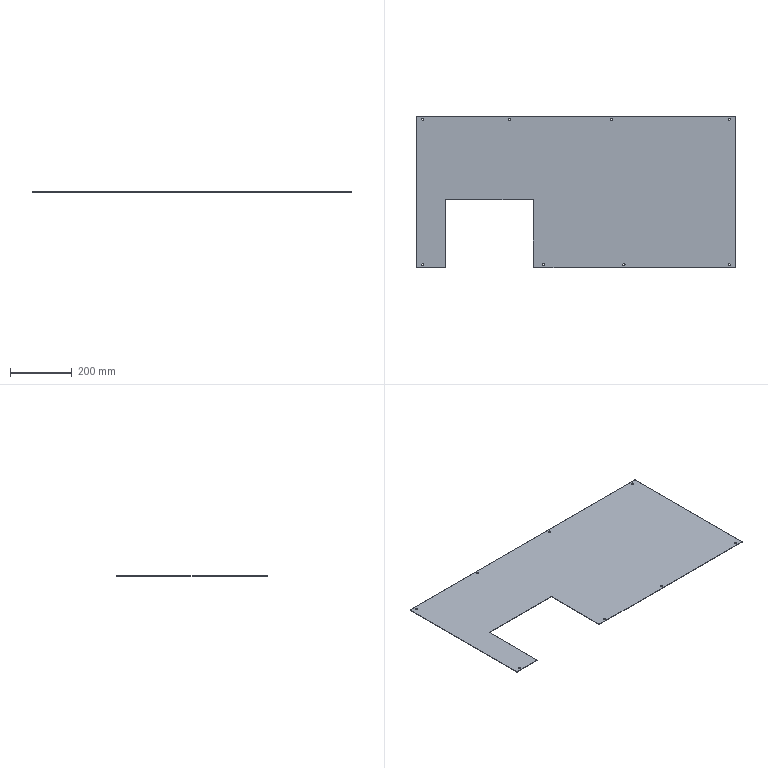Part | NX | 1 solid | 32 faces | box 1030 x 490 x 1.5 mm | volume 662860 mm3 | cylinder 22 | plane 10 | commonest cylinder face diameters 7 x16 4 x6
STEP:
#1=CARTESIAN_POINT('',(91.,0.,0.));
#2=VERTEX_POINT('',#1);
#3=CARTESIAN_POINT('',(2.,0.,0.));
#4=VERTEX_POINT('',#3);
#5=CARTESIAN_POINT('',(0.,0.,0.));
#6=DIRECTION('',(-1.,0.,0.));
#7=VECTOR('',#6,1000.);
#8=LINE('',#5,#7);
#9=EDGE_CURVE('',#2,#4,#8,.T.);
#10=ORIENTED_EDGE('',*,*,#9,.T.);
#11=CARTESIAN_POINT('',(0.,2.,0.));
#12=VERTEX_POINT('',#11);
#13=CARTESIAN_POINT('',(2.,2.,0.));
#14=DIRECTION('',(0.,0.,1.));
#15=DIRECTION('',(1.,0.,0.));
#16=AXIS2_PLACEMENT_3D('',#13,#14,#15);
#17=CIRCLE('',#16,2.);
#18=EDGE_CURVE('',#12,#4,#17,.T.);
#19=ORIENTED_EDGE('',*,*,#18,.F.);
#20=CARTESIAN_POINT('',(0.,488.,0.));
#21=VERTEX_POINT('',#20);
#22=CARTESIAN_POINT('',(0.,0.,0.));
#23=DIRECTION('',(0.,1.,0.));
#24=VECTOR('',#23,1000.);
#25=LINE('',#22,#24);
#26=EDGE_CURVE('',#12,#21,#25,.T.);
#27=ORIENTED_EDGE('',*,*,#26,.T.);
#28=CARTESIAN_POINT('',(2.,490.,0.));
#29=VERTEX_POINT('',#28);
#30=CARTESIAN_POINT('',(2.,488.,0.));
#31=DIRECTION('',(0.,0.,-1.));
#32=DIRECTION('',(-1.,0.,0.));
#33=AXIS2_PLACEMENT_3D('',#30,#31,#32);
#34=CIRCLE('',#33,2.);
#35=EDGE_CURVE('',#21,#29,#34,.T.);
#36=ORIENTED_EDGE('',*,*,#35,.T.);
#37=CARTESIAN_POINT('',(1028.,490.,0.));
#38=VERTEX_POINT('',#37);
#39=CARTESIAN_POINT('',(0.,490.,0.));
#40=DIRECTION('',(1.,0.,0.));
#41=VECTOR('',#40,1000.);
#42=LINE('',#39,#41);
#43=EDGE_CURVE('',#29,#38,#42,.T.);
#44=ORIENTED_EDGE('',*,*,#43,.T.);
#45=CARTESIAN_POINT('',(1030.,488.,0.));
#46=VERTEX_POINT('',#45);
#47=CARTESIAN_POINT('',(1028.,488.,0.));
#48=DIRECTION('',(0.,0.,-1.));
#49=DIRECTION('',(-1.,0.,0.));
#50=AXIS2_PLACEMENT_3D('',#47,#48,#49);
#51=CIRCLE('',#50,2.);
#52=EDGE_CURVE('',#38,#46,#51,.T.);
#53=ORIENTED_EDGE('',*,*,#52,.T.);
#54=CARTESIAN_POINT('',(1030.,2.,0.));
#55=VERTEX_POINT('',#54);
#56=CARTESIAN_POINT('',(1030.,0.,0.));
#57=DIRECTION('',(0.,-1.,0.));
#58=VECTOR('',#57,1000.);
#59=LINE('',#56,#58);
#60=EDGE_CURVE('',#46,#55,#59,.T.);
#61=ORIENTED_EDGE('',*,*,#60,.T.);
#62=CARTESIAN_POINT('',(1028.,0.,0.));
#63=VERTEX_POINT('',#62);
#64=CARTESIAN_POINT('',(1028.,2.,0.));
#65=DIRECTION('',(0.,0.,-1.));
#66=DIRECTION('',(-1.,0.,0.));
#67=AXIS2_PLACEMENT_3D('',#64,#65,#66);
#68=CIRCLE('',#67,2.);
#69=EDGE_CURVE('',#55,#63,#68,.T.);
#70=ORIENTED_EDGE('',*,*,#69,.T.);
#71=CARTESIAN_POINT('',(379.,0.,0.));
#72=VERTEX_POINT('',#71);
#73=CARTESIAN_POINT('',(0.,0.,0.));
#74=DIRECTION('',(-1.,0.,0.));
#75=VECTOR('',#74,1000.);
#76=LINE('',#73,#75);
#77=EDGE_CURVE('',#63,#72,#76,.T.);
#78=ORIENTED_EDGE('',*,*,#77,.T.);
#79=CARTESIAN_POINT('',(377.,2.,0.));
#80=VERTEX_POINT('',#79);
#81=CARTESIAN_POINT('',(379.,2.,0.));
#82=DIRECTION('',(0.,0.,-1.));
#83=DIRECTION('',(-1.,0.,0.));
#84=AXIS2_PLACEMENT_3D('',#81,#82,#83);
#85=CIRCLE('',#84,2.);
#86=EDGE_CURVE('',#72,#80,#85,.T.);
#87=ORIENTED_EDGE('',*,*,#86,.T.);
#88=CARTESIAN_POINT('',(377.,220.,0.));
#89=VERTEX_POINT('',#88);
#90=CARTESIAN_POINT('',(377.,0.,0.));
#91=DIRECTION('',(0.,-1.,0.));
#92=VECTOR('',#91,1000.);
#93=LINE('',#90,#92);
#94=EDGE_CURVE('',#89,#80,#93,.T.);
#95=ORIENTED_EDGE('',*,*,#94,.F.);
#96=CARTESIAN_POINT('',(93.,220.,0.));
#97=VERTEX_POINT('',#96);
#98=CARTESIAN_POINT('',(0.,220.,0.));
#99=DIRECTION('',(-1.,0.,0.));
#100=VECTOR('',#99,1000.);
#101=LINE('',#98,#100);
#102=EDGE_CURVE('',#89,#97,#101,.T.);
#103=ORIENTED_EDGE('',*,*,#102,.T.);
#104=CARTESIAN_POINT('',(93.,2.,0.));
#105=VERTEX_POINT('',#104);
#106=CARTESIAN_POINT('',(93.,0.,0.));
#107=DIRECTION('',(0.,1.,0.));
#108=VECTOR('',#107,1000.);
#109=LINE('',#106,#108);
#110=EDGE_CURVE('',#105,#97,#109,.T.);
#111=ORIENTED_EDGE('',*,*,#110,.F.);
#112=CARTESIAN_POINT('',(91.,2.,0.));
#113=DIRECTION('',(0.,0.,1.));
#114=DIRECTION('',(1.,0.,0.));
#115=AXIS2_PLACEMENT_3D('',#112,#113,#114);
#116=CIRCLE('',#115,2.);
#117=EDGE_CURVE('',#2,#105,#116,.T.);
#118=ORIENTED_EDGE('',*,*,#117,.F.);
#119=EDGE_LOOP('',(#10,#19,#27,#36,#44,#53,#61,#70,#78,#87,#95,#103,#111,#118));
#120=FACE_BOUND('',#119,.T.);
#121=CARTESIAN_POINT('',(1013.5,10.,0.));
#122=VERTEX_POINT('',#121);
#123=CARTESIAN_POINT('',(1006.5,10.,0.));
#124=VERTEX_POINT('',#123);
#125=CARTESIAN_POINT('',(1010.,10.,0.));
#126=DIRECTION('',(0.,0.,-1.));
#127=DIRECTION('',(-1.,0.,0.));
#128=AXIS2_PLACEMENT_3D('',#125,#126,#127);
#129=CIRCLE('',#128,3.5);
#130=EDGE_CURVE('',#122,#124,#129,.T.);
#131=ORIENTED_EDGE('',*,*,#130,.F.);
#132=CARTESIAN_POINT('',(1010.,10.,0.));
#133=DIRECTION('',(0.,0.,-1.));
#134=DIRECTION('',(-1.,0.,0.));
#135=AXIS2_PLACEMENT_3D('',#132,#133,#134);
#136=CIRCLE('',#135,3.5);
#137=EDGE_CURVE('',#124,#122,#136,.T.);
#138=ORIENTED_EDGE('',*,*,#137,.F.);
#139=EDGE_LOOP('',(#131,#138));
#140=FACE_BOUND('',#139,.T.);
#141=CARTESIAN_POINT('',(673.5,10.,0.));
#142=VERTEX_POINT('',#141);
#143=CARTESIAN_POINT('',(666.5,10.,0.));
#144=VERTEX_POINT('',#143);
#145=CARTESIAN_POINT('',(670.,10.,0.));
#146=DIRECTION('',(0.,0.,-1.));
#147=DIRECTION('',(-1.,0.,0.));
#148=AXIS2_PLACEMENT_3D('',#145,#146,#147);
#149=CIRCLE('',#148,3.5);
#150=EDGE_CURVE('',#142,#144,#149,.T.);
#151=ORIENTED_EDGE('',*,*,#150,.F.);
#152=CARTESIAN_POINT('',(670.,10.,0.));
#153=DIRECTION('',(0.,0.,-1.));
#154=DIRECTION('',(-1.,0.,0.));
#155=AXIS2_PLACEMENT_3D('',#152,#153,#154);
#156=CIRCLE('',#155,3.5);
#157=EDGE_CURVE('',#144,#142,#156,.T.);
#158=ORIENTED_EDGE('',*,*,#157,.F.);
#159=EDGE_LOOP('',(#151,#158));
#160=FACE_BOUND('',#159,.T.);
#161=CARTESIAN_POINT('',(413.5,10.,0.));
#162=VERTEX_POINT('',#161);
#163=CARTESIAN_POINT('',(406.5,10.,0.));
#164=VERTEX_POINT('',#163);
#165=CARTESIAN_POINT('',(410.,10.,0.));
#166=DIRECTION('',(0.,0.,-1.));
#167=DIRECTION('',(-1.,0.,0.));
#168=AXIS2_PLACEMENT_3D('',#165,#166,#167);
#169=CIRCLE('',#168,3.5);
#170=EDGE_CURVE('',#162,#164,#169,.T.);
#171=ORIENTED_EDGE('',*,*,#170,.F.);
#172=CARTESIAN_POINT('',(410.,10.,0.));
#173=DIRECTION('',(0.,0.,-1.));
#174=DIRECTION('',(-1.,0.,0.));
#175=AXIS2_PLACEMENT_3D('',#172,#173,#174);
#176=CIRCLE('',#175,3.5);
#177=EDGE_CURVE('',#164,#162,#176,.T.);
#178=ORIENTED_EDGE('',*,*,#177,.F.);
#179=EDGE_LOOP('',(#171,#178));
#180=FACE_BOUND('',#179,.T.);
#181=CARTESIAN_POINT('',(23.5,480.,0.));
#182=VERTEX_POINT('',#181);
#183=CARTESIAN_POINT('',(16.5,480.,0.));
#184=VERTEX_POINT('',#183);
#185=CARTESIAN_POINT('',(20.,480.,0.));
#186=DIRECTION('',(0.,0.,-1.));
#187=DIRECTION('',(-1.,0.,0.));
#188=AXIS2_PLACEMENT_3D('',#185,#186,#187);
#189=CIRCLE('',#188,3.5);
#190=EDGE_CURVE('',#182,#184,#189,.T.);
#191=ORIENTED_EDGE('',*,*,#190,.F.);
#192=CARTESIAN_POINT('',(20.,480.,0.));
#193=DIRECTION('',(0.,0.,-1.));
#194=DIRECTION('',(-1.,0.,0.));
#195=AXIS2_PLACEMENT_3D('',#192,#193,#194);
#196=CIRCLE('',#195,3.5);
#197=EDGE_CURVE('',#184,#182,#196,.T.);
#198=ORIENTED_EDGE('',*,*,#197,.F.);
#199=EDGE_LOOP('',(#191,#198));
#200=FACE_BOUND('',#199,.T.);
#201=CARTESIAN_POINT('',(1013.5,480.,0.));
#202=VERTEX_POINT('',#201);
#203=CARTESIAN_POINT('',(1006.5,480.,0.));
#204=VERTEX_POINT('',#203);
#205=CARTESIAN_POINT('',(1010.,480.,0.));
#206=DIRECTION('',(0.,0.,-1.));
#207=DIRECTION('',(-1.,0.,0.));
#208=AXIS2_PLACEMENT_3D('',#205,#206,#207);
#209=CIRCLE('',#208,3.5);
#210=EDGE_CURVE('',#202,#204,#209,.T.);
#211=ORIENTED_EDGE('',*,*,#210,.F.);
#212=CARTESIAN_POINT('',(1010.,480.,0.));
#213=DIRECTION('',(0.,0.,-1.));
#214=DIRECTION('',(-1.,0.,0.));
#215=AXIS2_PLACEMENT_3D('',#212,#213,#214);
#216=CIRCLE('',#215,3.5);
#217=EDGE_CURVE('',#204,#202,#216,.T.);
#218=ORIENTED_EDGE('',*,*,#217,.F.);
#219=EDGE_LOOP('',(#211,#218));
#220=FACE_BOUND('',#219,.T.);
#221=CARTESIAN_POINT('',(23.5,10.,0.));
#222=VERTEX_POINT('',#221);
#223=CARTESIAN_POINT('',(16.5,10.,0.));
#224=VERTEX_POINT('',#223);
#225=CARTESIAN_POINT('',(20.,10.,0.));
#226=DIRECTION('',(0.,0.,-1.));
#227=DIRECTION('',(-1.,0.,0.));
#228=AXIS2_PLACEMENT_3D('',#225,#226,#227);
#229=CIRCLE('',#228,3.5);
#230=EDGE_CURVE('',#222,#224,#229,.T.);
#231=ORIENTED_EDGE('',*,*,#230,.F.);
#232=CARTESIAN_POINT('',(20.,10.,0.));
#233=DIRECTION('',(0.,0.,-1.));
#234=DIRECTION('',(-1.,0.,0.));
#235=AXIS2_PLACEMENT_3D('',#232,#233,#234);
#236=CIRCLE('',#235,3.5);
#237=EDGE_CURVE('',#224,#222,#236,.T.);
#238=ORIENTED_EDGE('',*,*,#237,.F.);
#239=EDGE_LOOP('',(#231,#238));
#240=FACE_BOUND('',#239,.T.);
#241=CARTESIAN_POINT('',(633.5,480.,0.));
#242=VERTEX_POINT('',#241);
#243=CARTESIAN_POINT('',(626.5,480.,0.));
#244=VERTEX_POINT('',#243);
#245=CARTESIAN_POINT('',(630.,480.,0.));
#246=DIRECTION('',(0.,0.,-1.));
#247=DIRECTION('',(-1.,0.,0.));
#248=AXIS2_PLACEMENT_3D('',#245,#246,#247);
#249=CIRCLE('',#248,3.5);
#250=EDGE_CURVE('',#242,#244,#249,.T.);
#251=ORIENTED_EDGE('',*,*,#250,.F.);
#252=CARTESIAN_POINT('',(630.,480.,0.));
#253=DIRECTION('',(0.,0.,-1.));
#254=DIRECTION('',(-1.,0.,0.));
#255=AXIS2_PLACEMENT_3D('',#252,#253,#254);
#256=CIRCLE('',#255,3.5);
#257=EDGE_CURVE('',#244,#242,#256,.T.);
#258=ORIENTED_EDGE('',*,*,#257,.F.);
#259=EDGE_LOOP('',(#251,#258));
#260=FACE_BOUND('',#259,.T.);
#261=CARTESIAN_POINT('',(303.5,480.,0.));
#262=VERTEX_POINT('',#261);
#263=CARTESIAN_POINT('',(296.5,480.,0.));
#264=VERTEX_POINT('',#263);
#265=CARTESIAN_POINT('',(300.,480.,0.));
#266=DIRECTION('',(0.,0.,-1.));
#267=DIRECTION('',(-1.,0.,0.));
#268=AXIS2_PLACEMENT_3D('',#265,#266,#267);
#269=CIRCLE('',#268,3.5);
#270=EDGE_CURVE('',#262,#264,#269,.T.);
#271=ORIENTED_EDGE('',*,*,#270,.F.);
#272=CARTESIAN_POINT('',(300.,480.,0.));
#273=DIRECTION('',(0.,0.,-1.));
#274=DIRECTION('',(-1.,0.,0.));
#275=AXIS2_PLACEMENT_3D('',#272,#273,#274);
#276=CIRCLE('',#275,3.5);
#277=EDGE_CURVE('',#264,#262,#276,.T.);
#278=ORIENTED_EDGE('',*,*,#277,.F.);
#279=EDGE_LOOP('',(#271,#278));
#280=FACE_BOUND('',#279,.T.);
#281=CARTESIAN_POINT('',(0.,0.,0.));
#282=DIRECTION('',(0.,0.,1.));
#283=DIRECTION('',(1.,0.,0.));
#284=AXIS2_PLACEMENT_3D('',#281,#282,#283);
#285=PLANE('',#284);
#286=ADVANCED_FACE('',(#120,#140,#160,#180,#200,#220,#240,#260,#280),#285,.F.);
#287=CARTESIAN_POINT('',(2.,0.,1.5));
#288=VERTEX_POINT('',#287);
#289=CARTESIAN_POINT('',(2.,0.,0.));
#290=DIRECTION('',(0.,0.,1.));
#291=VECTOR('',#290,1000.);
#292=LINE('',#289,#291);
#293=EDGE_CURVE('',#4,#288,#292,.T.);
#294=ORIENTED_EDGE('',*,*,#293,.F.);
#295=ORIENTED_EDGE('',*,*,#9,.F.);
#296=CARTESIAN_POINT('',(91.,0.,1.5));
#297=VERTEX_POINT('',#296);
#298=CARTESIAN_POINT('',(91.,0.,0.));
#299=DIRECTION('',(0.,0.,1.));
#300=VECTOR('',#299,1000.);
#301=LINE('',#298,#300);
#302=EDGE_CURVE('',#2,#297,#301,.T.);
#303=ORIENTED_EDGE('',*,*,#302,.T.);
#304=CARTESIAN_POINT('',(0.,0.,1.5));
#305=DIRECTION('',(-1.,0.,0.));
#306=VECTOR('',#305,1000.);
#307=LINE('',#304,#306);
#308=EDGE_CURVE('',#297,#288,#307,.T.);
#309=ORIENTED_EDGE('',*,*,#308,.T.);
#310=EDGE_LOOP('',(#294,#295,#303,#309));
#311=FACE_BOUND('',#310,.T.);
#312=CARTESIAN_POINT('',(0.,0.,0.));
#313=DIRECTION('',(0.,-1.,0.));
#314=DIRECTION('',(0.,0.,-1.));
#315=AXIS2_PLACEMENT_3D('',#312,#313,#314);
#316=PLANE('',#315);
#317=ADVANCED_FACE('',(#311),#316,.T.);
#318=CARTESIAN_POINT('',(0.,488.,1.5));
#319=VERTEX_POINT('',#318);
#320=CARTESIAN_POINT('',(0.,488.,0.));
#321=DIRECTION('',(0.,0.,-1.));
#322=VECTOR('',#321,1000.);
#323=LINE('',#320,#322);
#324=EDGE_CURVE('',#319,#21,#323,.T.);
#325=ORIENTED_EDGE('',*,*,#324,.T.);
#326=ORIENTED_EDGE('',*,*,#26,.F.);
#327=CARTESIAN_POINT('',(0.,2.,1.5));
#328=VERTEX_POINT('',#327);
#329=CARTESIAN_POINT('',(0.,2.,0.));
#330=DIRECTION('',(0.,0.,1.));
#331=VECTOR('',#330,1000.);
#332=LINE('',#329,#331);
#333=EDGE_CURVE('',#12,#328,#332,.T.);
#334=ORIENTED_EDGE('',*,*,#333,.T.);
#335=CARTESIAN_POINT('',(0.,0.,1.5));
#336=DIRECTION('',(0.,1.,0.));
#337=VECTOR('',#336,1000.);
#338=LINE('',#335,#337);
#339=EDGE_CURVE('',#328,#319,#338,.T.);
#340=ORIENTED_EDGE('',*,*,#339,.T.);
#341=EDGE_LOOP('',(#325,#326,#334,#340));
#342=FACE_BOUND('',#341,.T.);
#343=CARTESIAN_POINT('',(0.,490.,0.));
#344=DIRECTION('',(-1.,0.,0.));
#345=DIRECTION('',(0.,0.,1.));
#346=AXIS2_PLACEMENT_3D('',#343,#344,#345);
#347=PLANE('',#346);
#348=ADVANCED_FACE('',(#342),#347,.T.);
#349=CARTESIAN_POINT('',(1028.,490.,1.5));
#350=VERTEX_POINT('',#349);
#351=CARTESIAN_POINT('',(1028.,490.,0.));
#352=DIRECTION('',(0.,0.,-1.));
#353=VECTOR('',#352,1000.);
#354=LINE('',#351,#353);
#355=EDGE_CURVE('',#350,#38,#354,.T.);
#356=ORIENTED_EDGE('',*,*,#355,.T.);
#357=ORIENTED_EDGE('',*,*,#43,.F.);
#358=CARTESIAN_POINT('',(2.,490.,1.5));
#359=VERTEX_POINT('',#358);
#360=CARTESIAN_POINT('',(2.,490.,0.));
#361=DIRECTION('',(0.,0.,-1.));
#362=VECTOR('',#361,1000.);
#363=LINE('',#360,#362);
#364=EDGE_CURVE('',#359,#29,#363,.T.);
#365=ORIENTED_EDGE('',*,*,#364,.F.);
#366=CARTESIAN_POINT('',(0.,490.,1.5));
#367=DIRECTION('',(1.,0.,0.));
#368=VECTOR('',#367,1000.);
#369=LINE('',#366,#368);
#370=EDGE_CURVE('',#359,#350,#369,.T.);
#371=ORIENTED_EDGE('',*,*,#370,.T.);
#372=EDGE_LOOP('',(#356,#357,#365,#371));
#373=FACE_BOUND('',#372,.T.);
#374=CARTESIAN_POINT('',(1030.,490.,0.));
#375=DIRECTION('',(0.,1.,0.));
#376=DIRECTION('',(1.,0.,0.));
#377=AXIS2_PLACEMENT_3D('',#374,#375,#376);
#378=PLANE('',#377);
#379=ADVANCED_FACE('',(#373),#378,.T.);
#380=CARTESIAN_POINT('',(1030.,2.,1.5));
#381=VERTEX_POINT('',#380);
#382=CARTESIAN_POINT('',(1030.,2.,0.));
#383=DIRECTION('',(0.,0.,-1.));
#384=VECTOR('',#383,1000.);
#385=LINE('',#382,#384);
#386=EDGE_CURVE('',#381,#55,#385,.T.);
#387=ORIENTED_EDGE('',*,*,#386,.T.);
#388=ORIENTED_EDGE('',*,*,#60,.F.);
#389=CARTESIAN_POINT('',(1030.,488.,1.5));
#390=VERTEX_POINT('',#389);
#391=CARTESIAN_POINT('',(1030.,488.,0.));
#392=DIRECTION('',(0.,0.,-1.));
#393=VECTOR('',#392,1000.);
#394=LINE('',#391,#393);
#395=EDGE_CURVE('',#390,#46,#394,.T.);
#396=ORIENTED_EDGE('',*,*,#395,.F.);
#397=CARTESIAN_POINT('',(1030.,0.,1.5));
#398=DIRECTION('',(0.,-1.,0.));
#399=VECTOR('',#398,1000.);
#400=LINE('',#397,#399);
#401=EDGE_CURVE('',#390,#381,#400,.T.);
#402=ORIENTED_EDGE('',*,*,#401,.T.);
#403=EDGE_LOOP('',(#387,#388,#396,#402));
#404=FACE_BOUND('',#403,.T.);
#405=CARTESIAN_POINT('',(1030.,0.,0.));
#406=DIRECTION('',(1.,0.,0.));
#407=DIRECTION('',(0.,1.,0.));
#408=AXIS2_PLACEMENT_3D('',#405,#406,#407);
#409=PLANE('',#408);
#410=ADVANCED_FACE('',(#404),#409,.T.);
#411=CARTESIAN_POINT('',(379.,0.,1.5));
#412=VERTEX_POINT('',#411);
#413=CARTESIAN_POINT('',(379.,0.,0.));
#414=DIRECTION('',(0.,0.,-1.));
#415=VECTOR('',#414,1000.);
#416=LINE('',#413,#415);
#417=EDGE_CURVE('',#412,#72,#416,.T.);
#418=ORIENTED_EDGE('',*,*,#417,.T.);
#419=ORIENTED_EDGE('',*,*,#77,.F.);
#420=CARTESIAN_POINT('',(1028.,0.,1.5));
#421=VERTEX_POINT('',#420);
#422=CARTESIAN_POINT('',(1028.,0.,0.));
#423=DIRECTION('',(0.,0.,-1.));
#424=VECTOR('',#423,1000.);
#425=LINE('',#422,#424);
#426=EDGE_CURVE('',#421,#63,#425,.T.);
#427=ORIENTED_EDGE('',*,*,#426,.F.);
#428=CARTESIAN_POINT('',(0.,0.,1.5));
#429=DIRECTION('',(-1.,0.,0.));
#430=VECTOR('',#429,1000.);
#431=LINE('',#428,#430);
#432=EDGE_CURVE('',#421,#412,#431,.T.);
#433=ORIENTED_EDGE('',*,*,#432,.T.);
#434=EDGE_LOOP('',(#418,#419,#427,#433));
#435=FACE_BOUND('',#434,.T.);
#436=CARTESIAN_POINT('',(545.,0.,0.));
#437=DIRECTION('',(0.,-1.,0.));
#438=DIRECTION('',(0.,0.,-1.));
#439=AXIS2_PLACEMENT_3D('',#436,#437,#438);
#440=PLANE('',#439);
#441=ADVANCED_FACE('',(#435),#440,.T.);
#442=ORIENTED_EDGE('',*,*,#94,.T.);
#443=CARTESIAN_POINT('',(377.,2.,1.5));
#444=VERTEX_POINT('',#443);
#445=CARTESIAN_POINT('',(377.,2.,0.));
#446=DIRECTION('',(0.,0.,-1.));
#447=VECTOR('',#446,1000.);
#448=LINE('',#445,#447);
#449=EDGE_CURVE('',#444,#80,#448,.T.);
#450=ORIENTED_EDGE('',*,*,#449,.F.);
#451=CARTESIAN_POINT('',(377.,220.,1.5));
#452=VERTEX_POINT('',#451);
#453=CARTESIAN_POINT('',(377.,0.,1.5));
#454=DIRECTION('',(0.,-1.,0.));
#455=VECTOR('',#454,1000.);
#456=LINE('',#453,#455);
#457=EDGE_CURVE('',#452,#444,#456,.T.);
#458=ORIENTED_EDGE('',*,*,#457,.F.);
#459=CARTESIAN_POINT('',(377.,220.,0.));
#460=DIRECTION('',(0.,0.,-1.));
#461=VECTOR('',#460,1000.);
#462=LINE('',#459,#461);
#463=EDGE_CURVE('',#452,#89,#462,.T.);
#464=ORIENTED_EDGE('',*,*,#463,.T.);
#465=EDGE_LOOP('',(#442,#450,#458,#464));
#466=FACE_BOUND('',#465,.T.);
#467=CARTESIAN_POINT('',(377.,220.,0.));
#468=DIRECTION('',(-1.,0.,0.));
#469=DIRECTION('',(0.,0.,1.));
#470=AXIS2_PLACEMENT_3D('',#467,#468,#469);
#471=PLANE('',#470);
#472=ADVANCED_FACE('',(#466),#471,.T.);
#473=ORIENTED_EDGE('',*,*,#102,.F.);
#474=ORIENTED_EDGE('',*,*,#463,.F.);
#475=CARTESIAN_POINT('',(93.,220.,1.5));
#476=VERTEX_POINT('',#475);
#477=CARTESIAN_POINT('',(0.,220.,1.5));
#478=DIRECTION('',(-1.,0.,0.));
#479=VECTOR('',#478,1000.);
#480=LINE('',#477,#479);
#481=EDGE_CURVE('',#452,#476,#480,.T.);
#482=ORIENTED_EDGE('',*,*,#481,.T.);
#483=CARTESIAN_POINT('',(93.,220.,0.));
#484=DIRECTION('',(0.,0.,1.));
#485=VECTOR('',#484,1000.);
#486=LINE('',#483,#485);
#487=EDGE_CURVE('',#97,#476,#486,.T.);
#488=ORIENTED_EDGE('',*,*,#487,.F.);
#489=EDGE_LOOP('',(#473,#474,#482,#488));
#490=FACE_BOUND('',#489,.T.);
#491=CARTESIAN_POINT('',(245.,220.,0.));
#492=DIRECTION('',(0.,-1.,0.));
#493=DIRECTION('',(0.,0.,-1.));
#494=AXIS2_PLACEMENT_3D('',#491,#492,#493);
#495=PLANE('',#494);
#496=ADVANCED_FACE('',(#490),#495,.T.);
#497=ORIENTED_EDGE('',*,*,#110,.T.);
#498=ORIENTED_EDGE('',*,*,#487,.T.);
#499=CARTESIAN_POINT('',(93.,2.,1.5));
#500=VERTEX_POINT('',#499);
#501=CARTESIAN_POINT('',(93.,0.,1.5));
#502=DIRECTION('',(0.,1.,0.));
#503=VECTOR('',#502,1000.);
#504=LINE('',#501,#503);
#505=EDGE_CURVE('',#500,#476,#504,.T.);
#506=ORIENTED_EDGE('',*,*,#505,.F.);
#507=CARTESIAN_POINT('',(93.,2.,0.));
#508=DIRECTION('',(0.,0.,1.));
#509=VECTOR('',#508,1000.);
#510=LINE('',#507,#509);
#511=EDGE_CURVE('',#105,#500,#510,.T.);
#512=ORIENTED_EDGE('',*,*,#511,.F.);
#513=EDGE_LOOP('',(#497,#498,#506,#512));
#514=FACE_BOUND('',#513,.T.);
#515=CARTESIAN_POINT('',(93.,0.,0.));
#516=DIRECTION('',(1.,0.,0.));
#517=DIRECTION('',(0.,1.,0.));
#518=AXIS2_PLACEMENT_3D('',#515,#516,#517);
#519=PLANE('',#518);
#520=ADVANCED_FACE('',(#514),#519,.T.);
#521=ORIENTED_EDGE('',*,*,#308,.F.);
#522=CARTESIAN_POINT('',(91.,2.,1.5));
#523=DIRECTION('',(0.,0.,1.));
#524=DIRECTION('',(1.,0.,0.));
#525=AXIS2_PLACEMENT_3D('',#522,#523,#524);
#526=CIRCLE('',#525,2.);
#527=EDGE_CURVE('',#297,#500,#526,.T.);
#528=ORIENTED_EDGE('',*,*,#527,.T.);
#529=ORIENTED_EDGE('',*,*,#505,.T.);
#530=ORIENTED_EDGE('',*,*,#481,.F.);
#531=ORIENTED_EDGE('',*,*,#457,.T.);
#532=CARTESIAN_POINT('',(379.,2.,1.5));
#533=DIRECTION('',(0.,0.,-1.));
#534=DIRECTION('',(-1.,0.,0.));
#535=AXIS2_PLACEMENT_3D('',#532,#533,#534);
#536=CIRCLE('',#535,2.);
#537=EDGE_CURVE('',#412,#444,#536,.T.);
#538=ORIENTED_EDGE('',*,*,#537,.F.);
#539=ORIENTED_EDGE('',*,*,#432,.F.);
#540=CARTESIAN_POINT('',(1028.,2.,1.5));
#541=DIRECTION('',(0.,0.,-1.));
#542=DIRECTION('',(-1.,0.,0.));
#543=AXIS2_PLACEMENT_3D('',#540,#541,#542);
#544=CIRCLE('',#543,2.);
#545=EDGE_CURVE('',#381,#421,#544,.T.);
#546=ORIENTED_EDGE('',*,*,#545,.F.);
#547=ORIENTED_EDGE('',*,*,#401,.F.);
#548=CARTESIAN_POINT('',(1028.,488.,1.5));
#549=DIRECTION('',(0.,0.,-1.));
#550=DIRECTION('',(-1.,0.,0.));
#551=AXIS2_PLACEMENT_3D('',#548,#549,#550);
#552=CIRCLE('',#551,2.);
#553=EDGE_CURVE('',#350,#390,#552,.T.);
#554=ORIENTED_EDGE('',*,*,#553,.F.);
#555=ORIENTED_EDGE('',*,*,#370,.F.);
#556=CARTESIAN_POINT('',(2.,488.,1.5));
#557=DIRECTION('',(0.,0.,-1.));
#558=DIRECTION('',(-1.,0.,0.));
#559=AXIS2_PLACEMENT_3D('',#556,#557,#558);
#560=CIRCLE('',#559,2.);
#561=EDGE_CURVE('',#319,#359,#560,.T.);
#562=ORIENTED_EDGE('',*,*,#561,.F.);
#563=ORIENTED_EDGE('',*,*,#339,.F.);
#564=CARTESIAN_POINT('',(2.,2.,1.5));
#565=DIRECTION('',(0.,0.,1.));
#566=DIRECTION('',(1.,0.,0.));
#567=AXIS2_PLACEMENT_3D('',#564,#565,#566);
#568=CIRCLE('',#567,2.);
#569=EDGE_CURVE('',#328,#288,#568,.T.);
#570=ORIENTED_EDGE('',*,*,#569,.T.);
#571=EDGE_LOOP('',(#521,#528,#529,#530,#531,#538,#539,#546,#547,#554,#555,#562,#563,#570));
#572=FACE_BOUND('',#571,.T.);
#573=CARTESIAN_POINT('',(1013.5,10.,1.5));
#574=VERTEX_POINT('',#573);
#575=CARTESIAN_POINT('',(1006.5,10.,1.5));
#576=VERTEX_POINT('',#575);
#577=CARTESIAN_POINT('',(1010.,10.,1.5));
#578=DIRECTION('',(0.,0.,-1.));
#579=DIRECTION('',(-1.,0.,0.));
#580=AXIS2_PLACEMENT_3D('',#577,#578,#579);
#581=CIRCLE('',#580,3.5);
#582=EDGE_CURVE('',#574,#576,#581,.T.);
#583=ORIENTED_EDGE('',*,*,#582,.T.);
#584=CARTESIAN_POINT('',(1010.,10.,1.5));
#585=DIRECTION('',(0.,0.,-1.));
#586=DIRECTION('',(-1.,0.,0.));
#587=AXIS2_PLACEMENT_3D('',#584,#585,#586);
#588=CIRCLE('',#587,3.5);
#589=EDGE_CURVE('',#576,#574,#588,.T.);
#590=ORIENTED_EDGE('',*,*,#589,.T.);
#591=EDGE_LOOP('',(#583,#590));
#592=FACE_BOUND('',#591,.T.);
#593=CARTESIAN_POINT('',(673.5,10.,1.5));
#594=VERTEX_POINT('',#593);
#595=CARTESIAN_POINT('',(666.5,10.,1.5));
#596=VERTEX_POINT('',#595);
#597=CARTESIAN_POINT('',(670.,10.,1.5));
#598=DIRECTION('',(0.,0.,-1.));
#599=DIRECTION('',(-1.,0.,0.));
#600=AXIS2_PLACEMENT_3D('',#597,#598,#599);
#601=CIRCLE('',#600,3.5);
#602=EDGE_CURVE('',#594,#596,#601,.T.);
#603=ORIENTED_EDGE('',*,*,#602,.T.);
#604=CARTESIAN_POINT('',(670.,10.,1.5));
#605=DIRECTION('',(0.,0.,-1.));
#606=DIRECTION('',(-1.,0.,0.));
#607=AXIS2_PLACEMENT_3D('',#604,#605,#606);
#608=CIRCLE('',#607,3.5);
#609=EDGE_CURVE('',#596,#594,#608,.T.);
#610=ORIENTED_EDGE('',*,*,#609,.T.);
#611=EDGE_LOOP('',(#603,#610));
#612=FACE_BOUND('',#611,.T.);
#613=CARTESIAN_POINT('',(413.5,10.,1.5));
#614=VERTEX_POINT('',#613);
#615=CARTESIAN_POINT('',(406.5,10.,1.5));
#616=VERTEX_POINT('',#615);
#617=CARTESIAN_POINT('',(410.,10.,1.5));
#618=DIRECTION('',(0.,0.,-1.));
#619=DIRECTION('',(-1.,0.,0.));
#620=AXIS2_PLACEMENT_3D('',#617,#618,#619);
#621=CIRCLE('',#620,3.5);
#622=EDGE_CURVE('',#614,#616,#621,.T.);
#623=ORIENTED_EDGE('',*,*,#622,.T.);
#624=CARTESIAN_POINT('',(410.,10.,1.5));
#625=DIRECTION('',(0.,0.,-1.));
#626=DIRECTION('',(-1.,0.,0.));
#627=AXIS2_PLACEMENT_3D('',#624,#625,#626);
#628=CIRCLE('',#627,3.5);
#629=EDGE_CURVE('',#616,#614,#628,.T.);
#630=ORIENTED_EDGE('',*,*,#629,.T.);
#631=EDGE_LOOP('',(#623,#630));
#632=FACE_BOUND('',#631,.T.);
#633=CARTESIAN_POINT('',(23.5,480.,1.5));
#634=VERTEX_POINT('',#633);
#635=CARTESIAN_POINT('',(16.5,480.,1.5));
#636=VERTEX_POINT('',#635);
#637=CARTESIAN_POINT('',(20.,480.,1.5));
#638=DIRECTION('',(0.,0.,-1.));
#639=DIRECTION('',(-1.,0.,0.));
#640=AXIS2_PLACEMENT_3D('',#637,#638,#639);
#641=CIRCLE('',#640,3.5);
#642=EDGE_CURVE('',#634,#636,#641,.T.);
#643=ORIENTED_EDGE('',*,*,#642,.T.);
#644=CARTESIAN_POINT('',(20.,480.,1.5));
#645=DIRECTION('',(0.,0.,-1.));
#646=DIRECTION('',(-1.,0.,0.));
#647=AXIS2_PLACEMENT_3D('',#644,#645,#646);
#648=CIRCLE('',#647,3.5);
#649=EDGE_CURVE('',#636,#634,#648,.T.);
#650=ORIENTED_EDGE('',*,*,#649,.T.);
#651=EDGE_LOOP('',(#643,#650));
#652=FACE_BOUND('',#651,.T.);
#653=CARTESIAN_POINT('',(1013.5,480.,1.5));
#654=VERTEX_POINT('',#653);
#655=CARTESIAN_POINT('',(1006.5,480.,1.5));
#656=VERTEX_POINT('',#655);
#657=CARTESIAN_POINT('',(1010.,480.,1.5));
#658=DIRECTION('',(0.,0.,-1.));
#659=DIRECTION('',(-1.,0.,0.));
#660=AXIS2_PLACEMENT_3D('',#657,#658,#659);
#661=CIRCLE('',#660,3.5);
#662=EDGE_CURVE('',#654,#656,#661,.T.);
#663=ORIENTED_EDGE('',*,*,#662,.T.);
#664=CARTESIAN_POINT('',(1010.,480.,1.5));
#665=DIRECTION('',(0.,0.,-1.));
#666=DIRECTION('',(-1.,0.,0.));
#667=AXIS2_PLACEMENT_3D('',#664,#665,#666);
#668=CIRCLE('',#667,3.5);
#669=EDGE_CURVE('',#656,#654,#668,.T.);
#670=ORIENTED_EDGE('',*,*,#669,.T.);
#671=EDGE_LOOP('',(#663,#670));
#672=FACE_BOUND('',#671,.T.);
#673=CARTESIAN_POINT('',(23.5,10.,1.5));
#674=VERTEX_POINT('',#673);
#675=CARTESIAN_POINT('',(16.5,10.,1.5));
#676=VERTEX_POINT('',#675);
#677=CARTESIAN_POINT('',(20.,10.,1.5));
#678=DIRECTION('',(0.,0.,-1.));
#679=DIRECTION('',(-1.,0.,0.));
#680=AXIS2_PLACEMENT_3D('',#677,#678,#679);
#681=CIRCLE('',#680,3.5);
#682=EDGE_CURVE('',#674,#676,#681,.T.);
#683=ORIENTED_EDGE('',*,*,#682,.T.);
#684=CARTESIAN_POINT('',(20.,10.,1.5));
#685=DIRECTION('',(0.,0.,-1.));
#686=DIRECTION('',(-1.,0.,0.));
#687=AXIS2_PLACEMENT_3D('',#684,#685,#686);
#688=CIRCLE('',#687,3.5);
#689=EDGE_CURVE('',#676,#674,#688,.T.);
#690=ORIENTED_EDGE('',*,*,#689,.T.);
#691=EDGE_LOOP('',(#683,#690));
#692=FACE_BOUND('',#691,.T.);
#693=CARTESIAN_POINT('',(633.5,480.,1.5));
#694=VERTEX_POINT('',#693);
#695=CARTESIAN_POINT('',(626.5,480.,1.5));
#696=VERTEX_POINT('',#695);
#697=CARTESIAN_POINT('',(630.,480.,1.5));
#698=DIRECTION('',(0.,0.,-1.));
#699=DIRECTION('',(-1.,0.,0.));
#700=AXIS2_PLACEMENT_3D('',#697,#698,#699);
#701=CIRCLE('',#700,3.5);
#702=EDGE_CURVE('',#694,#696,#701,.T.);
#703=ORIENTED_EDGE('',*,*,#702,.T.);
#704=CARTESIAN_POINT('',(630.,480.,1.5));
#705=DIRECTION('',(0.,0.,-1.));
#706=DIRECTION('',(-1.,0.,0.));
#707=AXIS2_PLACEMENT_3D('',#704,#705,#706);
#708=CIRCLE('',#707,3.5);
#709=EDGE_CURVE('',#696,#694,#708,.T.);
#710=ORIENTED_EDGE('',*,*,#709,.T.);
#711=EDGE_LOOP('',(#703,#710));
#712=FACE_BOUND('',#711,.T.);
#713=CARTESIAN_POINT('',(303.5,480.,1.5));
#714=VERTEX_POINT('',#713);
#715=CARTESIAN_POINT('',(296.5,480.,1.5));
#716=VERTEX_POINT('',#715);
#717=CARTESIAN_POINT('',(300.,480.,1.5));
#718=DIRECTION('',(0.,0.,-1.));
#719=DIRECTION('',(-1.,0.,0.));
#720=AXIS2_PLACEMENT_3D('',#717,#718,#719);
#721=CIRCLE('',#720,3.5);
#722=EDGE_CURVE('',#714,#716,#721,.T.);
#723=ORIENTED_EDGE('',*,*,#722,.T.);
#724=CARTESIAN_POINT('',(300.,480.,1.5));
#725=DIRECTION('',(0.,0.,-1.));
#726=DIRECTION('',(-1.,0.,0.));
#727=AXIS2_PLACEMENT_3D('',#724,#725,#726);
#728=CIRCLE('',#727,3.5);
#729=EDGE_CURVE('',#716,#714,#728,.T.);
#730=ORIENTED_EDGE('',*,*,#729,.T.);
#731=EDGE_LOOP('',(#723,#730));
#732=FACE_BOUND('',#731,.T.);
#733=CARTESIAN_POINT('',(0.,0.,1.5));
#734=DIRECTION('',(0.,0.,1.));
#735=DIRECTION('',(1.,0.,0.));
#736=AXIS2_PLACEMENT_3D('',#733,#734,#735);
#737=PLANE('',#736);
#738=ADVANCED_FACE('',(#572,#592,#612,#632,#652,#672,#692,#712,#732),#737,.T.);
#739=ORIENTED_EDGE('',*,*,#130,.T.);
#740=CARTESIAN_POINT('',(1006.5,10.,1.5));
#741=DIRECTION('',(0.,0.,-1.));
#742=VECTOR('',#741,1000.);
#743=LINE('',#740,#742);
#744=EDGE_CURVE('',#124,#576,#743,.F.);
#745=ORIENTED_EDGE('',*,*,#744,.T.);
#746=ORIENTED_EDGE('',*,*,#582,.F.);
#747=CARTESIAN_POINT('',(1013.5,10.,1.5));
#748=DIRECTION('',(0.,0.,-1.));
#749=VECTOR('',#748,1000.);
#750=LINE('',#747,#749);
#751=EDGE_CURVE('',#122,#574,#750,.F.);
#752=ORIENTED_EDGE('',*,*,#751,.F.);
#753=EDGE_LOOP('',(#739,#745,#746,#752));
#754=FACE_BOUND('',#753,.T.);
#755=CARTESIAN_POINT('',(1010.,10.,1.5));
#756=DIRECTION('',(0.,0.,-1.));
#757=DIRECTION('',(-1.,0.,0.));
#758=AXIS2_PLACEMENT_3D('',#755,#756,#757);
#759=CYLINDRICAL_SURFACE('',#758,3.5);
#760=ADVANCED_FACE('',(#754),#759,.F.);
#761=ORIENTED_EDGE('',*,*,#702,.F.);
#762=CARTESIAN_POINT('',(633.5,480.,1.5));
#763=DIRECTION('',(0.,0.,-1.));
#764=VECTOR('',#763,1000.);
#765=LINE('',#762,#764);
#766=EDGE_CURVE('',#242,#694,#765,.F.);
#767=ORIENTED_EDGE('',*,*,#766,.F.);
#768=ORIENTED_EDGE('',*,*,#250,.T.);
#769=CARTESIAN_POINT('',(626.5,480.,1.5));
#770=DIRECTION('',(0.,0.,-1.));
#771=VECTOR('',#770,1000.);
#772=LINE('',#769,#771);
#773=EDGE_CURVE('',#244,#696,#772,.F.);
#774=ORIENTED_EDGE('',*,*,#773,.T.);
#775=EDGE_LOOP('',(#761,#767,#768,#774));
#776=FACE_BOUND('',#775,.T.);
#777=CARTESIAN_POINT('',(630.,480.,1.5));
#778=DIRECTION('',(0.,0.,-1.));
#779=DIRECTION('',(-1.,0.,0.));
#780=AXIS2_PLACEMENT_3D('',#777,#778,#779);
#781=CYLINDRICAL_SURFACE('',#780,3.5);
#782=ADVANCED_FACE('',(#776),#781,.F.);
#783=ORIENTED_EDGE('',*,*,#602,.F.);
#784=CARTESIAN_POINT('',(673.5,10.,1.5));
#785=DIRECTION('',(0.,0.,-1.));
#786=VECTOR('',#785,1000.);
#787=LINE('',#784,#786);
#788=EDGE_CURVE('',#142,#594,#787,.F.);
#789=ORIENTED_EDGE('',*,*,#788,.F.);
#790=ORIENTED_EDGE('',*,*,#150,.T.);
#791=CARTESIAN_POINT('',(666.5,10.,1.5));
#792=DIRECTION('',(0.,0.,-1.));
#793=VECTOR('',#792,1000.);
#794=LINE('',#791,#793);
#795=EDGE_CURVE('',#144,#596,#794,.F.);
#796=ORIENTED_EDGE('',*,*,#795,.T.);
#797=EDGE_LOOP('',(#783,#789,#790,#796));
#798=FACE_BOUND('',#797,.T.);
#799=CARTESIAN_POINT('',(670.,10.,1.5));
#800=DIRECTION('',(0.,0.,-1.));
#801=DIRECTION('',(-1.,0.,0.));
#802=AXIS2_PLACEMENT_3D('',#799,#800,#801);
#803=CYLINDRICAL_SURFACE('',#802,3.5);
#804=ADVANCED_FACE('',(#798),#803,.F.);
#805=ORIENTED_EDGE('',*,*,#662,.F.);
#806=CARTESIAN_POINT('',(1013.5,480.,1.5));
#807=DIRECTION('',(0.,0.,-1.));
#808=VECTOR('',#807,1000.);
#809=LINE('',#806,#808);
#810=EDGE_CURVE('',#202,#654,#809,.F.);
#811=ORIENTED_EDGE('',*,*,#810,.F.);
#812=ORIENTED_EDGE('',*,*,#210,.T.);
#813=CARTESIAN_POINT('',(1006.5,480.,1.5));
#814=DIRECTION('',(0.,0.,-1.));
#815=VECTOR('',#814,1000.);
#816=LINE('',#813,#815);
#817=EDGE_CURVE('',#204,#656,#816,.F.);
#818=ORIENTED_EDGE('',*,*,#817,.T.);
#819=EDGE_LOOP('',(#805,#811,#812,#818));
#820=FACE_BOUND('',#819,.T.);
#821=CARTESIAN_POINT('',(1010.,480.,1.5));
#822=DIRECTION('',(0.,0.,-1.));
#823=DIRECTION('',(-1.,0.,0.));
#824=AXIS2_PLACEMENT_3D('',#821,#822,#823);
#825=CYLINDRICAL_SURFACE('',#824,3.5);
#826=ADVANCED_FACE('',(#820),#825,.F.);
#827=ORIENTED_EDGE('',*,*,#622,.F.);
#828=CARTESIAN_POINT('',(413.5,10.,1.5));
#829=DIRECTION('',(0.,0.,-1.));
#830=VECTOR('',#829,1000.);
#831=LINE('',#828,#830);
#832=EDGE_CURVE('',#162,#614,#831,.F.);
#833=ORIENTED_EDGE('',*,*,#832,.F.);
#834=ORIENTED_EDGE('',*,*,#170,.T.);
#835=CARTESIAN_POINT('',(406.5,10.,1.5));
#836=DIRECTION('',(0.,0.,-1.));
#837=VECTOR('',#836,1000.);
#838=LINE('',#835,#837);
#839=EDGE_CURVE('',#164,#616,#838,.F.);
#840=ORIENTED_EDGE('',*,*,#839,.T.);
#841=EDGE_LOOP('',(#827,#833,#834,#840));
#842=FACE_BOUND('',#841,.T.);
#843=CARTESIAN_POINT('',(410.,10.,1.5));
#844=DIRECTION('',(0.,0.,-1.));
#845=DIRECTION('',(-1.,0.,0.));
#846=AXIS2_PLACEMENT_3D('',#843,#844,#845);
#847=CYLINDRICAL_SURFACE('',#846,3.5);
#848=ADVANCED_FACE('',(#842),#847,.F.);
#849=ORIENTED_EDGE('',*,*,#682,.F.);
#850=CARTESIAN_POINT('',(23.5,10.,1.5));
#851=DIRECTION('',(0.,0.,-1.));
#852=VECTOR('',#851,1000.);
#853=LINE('',#850,#852);
#854=EDGE_CURVE('',#222,#674,#853,.F.);
#855=ORIENTED_EDGE('',*,*,#854,.F.);
#856=ORIENTED_EDGE('',*,*,#230,.T.);
#857=CARTESIAN_POINT('',(16.5,10.,1.5));
#858=DIRECTION('',(0.,0.,-1.));
#859=VECTOR('',#858,1000.);
#860=LINE('',#857,#859);
#861=EDGE_CURVE('',#224,#676,#860,.F.);
#862=ORIENTED_EDGE('',*,*,#861,.T.);
#863=EDGE_LOOP('',(#849,#855,#856,#862));
#864=FACE_BOUND('',#863,.T.);
#865=CARTESIAN_POINT('',(20.,10.,1.5));
#866=DIRECTION('',(0.,0.,-1.));
#867=DIRECTION('',(-1.,0.,0.));
#868=AXIS2_PLACEMENT_3D('',#865,#866,#867);
#869=CYLINDRICAL_SURFACE('',#868,3.5);
#870=ADVANCED_FACE('',(#864),#869,.F.);
#871=ORIENTED_EDGE('',*,*,#642,.F.);
#872=CARTESIAN_POINT('',(23.5,480.,1.5));
#873=DIRECTION('',(0.,0.,-1.));
#874=VECTOR('',#873,1000.);
#875=LINE('',#872,#874);
#876=EDGE_CURVE('',#182,#634,#875,.F.);
#877=ORIENTED_EDGE('',*,*,#876,.F.);
#878=ORIENTED_EDGE('',*,*,#190,.T.);
#879=CARTESIAN_POINT('',(16.5,480.,1.5));
#880=DIRECTION('',(0.,0.,-1.));
#881=VECTOR('',#880,1000.);
#882=LINE('',#879,#881);
#883=EDGE_CURVE('',#184,#636,#882,.F.);
#884=ORIENTED_EDGE('',*,*,#883,.T.);
#885=EDGE_LOOP('',(#871,#877,#878,#884));
#886=FACE_BOUND('',#885,.T.);
#887=CARTESIAN_POINT('',(20.,480.,1.5));
#888=DIRECTION('',(0.,0.,-1.));
#889=DIRECTION('',(-1.,0.,0.));
#890=AXIS2_PLACEMENT_3D('',#887,#888,#889);
#891=CYLINDRICAL_SURFACE('',#890,3.5);
#892=ADVANCED_FACE('',(#886),#891,.F.);
#893=ORIENTED_EDGE('',*,*,#722,.F.);
#894=CARTESIAN_POINT('',(303.5,480.,1.5));
#895=DIRECTION('',(0.,0.,-1.));
#896=VECTOR('',#895,1000.);
#897=LINE('',#894,#896);
#898=EDGE_CURVE('',#262,#714,#897,.F.);
#899=ORIENTED_EDGE('',*,*,#898,.F.);
#900=ORIENTED_EDGE('',*,*,#270,.T.);
#901=CARTESIAN_POINT('',(296.5,480.,1.5));
#902=DIRECTION('',(0.,0.,-1.));
#903=VECTOR('',#902,1000.);
#904=LINE('',#901,#903);
#905=EDGE_CURVE('',#264,#716,#904,.F.);
#906=ORIENTED_EDGE('',*,*,#905,.T.);
#907=EDGE_LOOP('',(#893,#899,#900,#906));
#908=FACE_BOUND('',#907,.T.);
#909=CARTESIAN_POINT('',(300.,480.,1.5));
#910=DIRECTION('',(0.,0.,-1.));
#911=DIRECTION('',(-1.,0.,0.));
#912=AXIS2_PLACEMENT_3D('',#909,#910,#911);
#913=CYLINDRICAL_SURFACE('',#912,3.5);
#914=ADVANCED_FACE('',(#908),#913,.F.);
#915=ORIENTED_EDGE('',*,*,#355,.F.);
#916=ORIENTED_EDGE('',*,*,#553,.T.);
#917=ORIENTED_EDGE('',*,*,#395,.T.);
#918=ORIENTED_EDGE('',*,*,#52,.F.);
#919=EDGE_LOOP('',(#915,#916,#917,#918));
#920=FACE_BOUND('',#919,.T.);
#921=CARTESIAN_POINT('',(1028.,488.,0.));
#922=DIRECTION('',(0.,0.,-1.));
#923=DIRECTION('',(-1.,0.,0.));
#924=AXIS2_PLACEMENT_3D('',#921,#922,#923);
#925=CYLINDRICAL_SURFACE('',#924,2.);
#926=ADVANCED_FACE('',(#920),#925,.T.);
#927=ORIENTED_EDGE('',*,*,#386,.F.);
#928=ORIENTED_EDGE('',*,*,#545,.T.);
#929=ORIENTED_EDGE('',*,*,#426,.T.);
#930=ORIENTED_EDGE('',*,*,#69,.F.);
#931=EDGE_LOOP('',(#927,#928,#929,#930));
#932=FACE_BOUND('',#931,.T.);
#933=CARTESIAN_POINT('',(1028.,2.,0.));
#934=DIRECTION('',(0.,0.,-1.));
#935=DIRECTION('',(-1.,0.,0.));
#936=AXIS2_PLACEMENT_3D('',#933,#934,#935);
#937=CYLINDRICAL_SURFACE('',#936,2.);
#938=ADVANCED_FACE('',(#932),#937,.T.);
#939=ORIENTED_EDGE('',*,*,#417,.F.);
#940=ORIENTED_EDGE('',*,*,#537,.T.);
#941=ORIENTED_EDGE('',*,*,#449,.T.);
#942=ORIENTED_EDGE('',*,*,#86,.F.);
#943=EDGE_LOOP('',(#939,#940,#941,#942));
#944=FACE_BOUND('',#943,.T.);
#945=CARTESIAN_POINT('',(379.,2.,0.));
#946=DIRECTION('',(0.,0.,-1.));
#947=DIRECTION('',(-1.,0.,0.));
#948=AXIS2_PLACEMENT_3D('',#945,#946,#947);
#949=CYLINDRICAL_SURFACE('',#948,2.);
#950=ADVANCED_FACE('',(#944),#949,.T.);
#951=ORIENTED_EDGE('',*,*,#302,.F.);
#952=ORIENTED_EDGE('',*,*,#117,.T.);
#953=ORIENTED_EDGE('',*,*,#511,.T.);
#954=ORIENTED_EDGE('',*,*,#527,.F.);
#955=EDGE_LOOP('',(#951,#952,#953,#954));
#956=FACE_BOUND('',#955,.T.);
#957=CARTESIAN_POINT('',(91.,2.,0.));
#958=DIRECTION('',(0.,0.,1.));
#959=DIRECTION('',(1.,0.,0.));
#960=AXIS2_PLACEMENT_3D('',#957,#958,#959);
#961=CYLINDRICAL_SURFACE('',#960,2.);
#962=ADVANCED_FACE('',(#956),#961,.T.);
#963=ORIENTED_EDGE('',*,*,#293,.T.);
#964=ORIENTED_EDGE('',*,*,#569,.F.);
#965=ORIENTED_EDGE('',*,*,#333,.F.);
#966=ORIENTED_EDGE('',*,*,#18,.T.);
#967=EDGE_LOOP('',(#963,#964,#965,#966));
#968=FACE_BOUND('',#967,.T.);
#969=CARTESIAN_POINT('',(2.,2.,0.));
#970=DIRECTION('',(0.,0.,1.));
#971=DIRECTION('',(1.,0.,0.));
#972=AXIS2_PLACEMENT_3D('',#969,#970,#971);
#973=CYLINDRICAL_SURFACE('',#972,2.);
#974=ADVANCED_FACE('',(#968),#973,.T.);
#975=ORIENTED_EDGE('',*,*,#324,.F.);
#976=ORIENTED_EDGE('',*,*,#561,.T.);
#977=ORIENTED_EDGE('',*,*,#364,.T.);
#978=ORIENTED_EDGE('',*,*,#35,.F.);
#979=EDGE_LOOP('',(#975,#976,#977,#978));
#980=FACE_BOUND('',#979,.T.);
#981=CARTESIAN_POINT('',(2.,488.,0.));
#982=DIRECTION('',(0.,0.,-1.));
#983=DIRECTION('',(-1.,0.,0.));
#984=AXIS2_PLACEMENT_3D('',#981,#982,#983);
#985=CYLINDRICAL_SURFACE('',#984,2.);
#986=ADVANCED_FACE('',(#980),#985,.T.);
#987=ORIENTED_EDGE('',*,*,#861,.F.);
#988=ORIENTED_EDGE('',*,*,#237,.T.);
#989=ORIENTED_EDGE('',*,*,#854,.T.);
#990=ORIENTED_EDGE('',*,*,#689,.F.);
#991=EDGE_LOOP('',(#987,#988,#989,#990));
#992=FACE_BOUND('',#991,.T.);
#993=CARTESIAN_POINT('',(20.,10.,1.5));
#994=DIRECTION('',(0.,0.,-1.));
#995=DIRECTION('',(-1.,0.,0.));
#996=AXIS2_PLACEMENT_3D('',#993,#994,#995);
#997=CYLINDRICAL_SURFACE('',#996,3.5);
#998=ADVANCED_FACE('',(#992),#997,.F.);
#999=ORIENTED_EDGE('',*,*,#817,.F.);
#1000=ORIENTED_EDGE('',*,*,#217,.T.);
#1001=ORIENTED_EDGE('',*,*,#810,.T.);
#1002=ORIENTED_EDGE('',*,*,#669,.F.);
#1003=EDGE_LOOP('',(#999,#1000,#1001,#1002));
#1004=FACE_BOUND('',#1003,.T.);
#1005=CARTESIAN_POINT('',(1010.,480.,1.5));
#1006=DIRECTION('',(0.,0.,-1.));
#1007=DIRECTION('',(-1.,0.,0.));
#1008=AXIS2_PLACEMENT_3D('',#1005,#1006,#1007);
#1009=CYLINDRICAL_SURFACE('',#1008,3.5);
#1010=ADVANCED_FACE('',(#1004),#1009,.F.);
#1011=ORIENTED_EDGE('',*,*,#883,.F.);
#1012=ORIENTED_EDGE('',*,*,#197,.T.);
#1013=ORIENTED_EDGE('',*,*,#876,.T.);
#1014=ORIENTED_EDGE('',*,*,#649,.F.);
#1015=EDGE_LOOP('',(#1011,#1012,#1013,#1014));
#1016=FACE_BOUND('',#1015,.T.);
#1017=CARTESIAN_POINT('',(20.,480.,1.5));
#1018=DIRECTION('',(0.,0.,-1.));
#1019=DIRECTION('',(-1.,0.,0.));
#1020=AXIS2_PLACEMENT_3D('',#1017,#1018,#1019);
#1021=CYLINDRICAL_SURFACE('',#1020,3.5);
#1022=ADVANCED_FACE('',(#1016),#1021,.F.);
#1023=ORIENTED_EDGE('',*,*,#839,.F.);
#1024=ORIENTED_EDGE('',*,*,#177,.T.);
#1025=ORIENTED_EDGE('',*,*,#832,.T.);
#1026=ORIENTED_EDGE('',*,*,#629,.F.);
#1027=EDGE_LOOP('',(#1023,#1024,#1025,#1026));
#1028=FACE_BOUND('',#1027,.T.);
#1029=CARTESIAN_POINT('',(410.,10.,1.5));
#1030=DIRECTION('',(0.,0.,-1.));
#1031=DIRECTION('',(-1.,0.,0.));
#1032=AXIS2_PLACEMENT_3D('',#1029,#1030,#1031);
#1033=CYLINDRICAL_SURFACE('',#1032,3.5);
#1034=ADVANCED_FACE('',(#1028),#1033,.F.);
#1035=ORIENTED_EDGE('',*,*,#795,.F.);
#1036=ORIENTED_EDGE('',*,*,#157,.T.);
#1037=ORIENTED_EDGE('',*,*,#788,.T.);
#1038=ORIENTED_EDGE('',*,*,#609,.F.);
#1039=EDGE_LOOP('',(#1035,#1036,#1037,#1038));
#1040=FACE_BOUND('',#1039,.T.);
#1041=CARTESIAN_POINT('',(670.,10.,1.5));
#1042=DIRECTION('',(0.,0.,-1.));
#1043=DIRECTION('',(-1.,0.,0.));
#1044=AXIS2_PLACEMENT_3D('',#1041,#1042,#1043);
#1045=CYLINDRICAL_SURFACE('',#1044,3.5);
#1046=ADVANCED_FACE('',(#1040),#1045,.F.);
#1047=ORIENTED_EDGE('',*,*,#905,.F.);
#1048=ORIENTED_EDGE('',*,*,#277,.T.);
#1049=ORIENTED_EDGE('',*,*,#898,.T.);
#1050=ORIENTED_EDGE('',*,*,#729,.F.);
#1051=EDGE_LOOP('',(#1047,#1048,#1049,#1050));
#1052=FACE_BOUND('',#1051,.T.);
#1053=CARTESIAN_POINT('',(300.,480.,1.5));
#1054=DIRECTION('',(0.,0.,-1.));
#1055=DIRECTION('',(-1.,0.,0.));
#1056=AXIS2_PLACEMENT_3D('',#1053,#1054,#1055);
#1057=CYLINDRICAL_SURFACE('',#1056,3.5);
#1058=ADVANCED_FACE('',(#1052),#1057,.F.);
#1059=ORIENTED_EDGE('',*,*,#773,.F.);
#1060=ORIENTED_EDGE('',*,*,#257,.T.);
#1061=ORIENTED_EDGE('',*,*,#766,.T.);
#1062=ORIENTED_EDGE('',*,*,#709,.F.);
#1063=EDGE_LOOP('',(#1059,#1060,#1061,#1062));
#1064=FACE_BOUND('',#1063,.T.);
#1065=CARTESIAN_POINT('',(630.,480.,1.5));
#1066=DIRECTION('',(0.,0.,-1.));
#1067=DIRECTION('',(-1.,0.,0.));
#1068=AXIS2_PLACEMENT_3D('',#1065,#1066,#1067);
#1069=CYLINDRICAL_SURFACE('',#1068,3.5);
#1070=ADVANCED_FACE('',(#1064),#1069,.F.);
#1071=ORIENTED_EDGE('',*,*,#744,.F.);
#1072=ORIENTED_EDGE('',*,*,#137,.T.);
#1073=ORIENTED_EDGE('',*,*,#751,.T.);
#1074=ORIENTED_EDGE('',*,*,#589,.F.);
#1075=EDGE_LOOP('',(#1071,#1072,#1073,#1074));
#1076=FACE_BOUND('',#1075,.T.);
#1077=CARTESIAN_POINT('',(1010.,10.,1.5));
#1078=DIRECTION('',(0.,0.,-1.));
#1079=DIRECTION('',(-1.,0.,0.));
#1080=AXIS2_PLACEMENT_3D('',#1077,#1078,#1079);
#1081=CYLINDRICAL_SURFACE('',#1080,3.5);
#1082=ADVANCED_FACE('',(#1076),#1081,.F.);
#1083=CLOSED_SHELL('',(#286,#317,#348,#379,#410,#441,#472,#496,#520,#738,#760,#782,#804,#826,#848,#870,#892,#914,#926,#938,#950,#962,#974,#986,#998,#1010,#1022,#1034,#1046,#1058,#1070,#1082));
#1084=MANIFOLD_SOLID_BREP('',#1083);
#1085=(LENGTH_UNIT()NAMED_UNIT(*)SI_UNIT(.MILLI.,.METRE.));
#1086=UNCERTAINTY_MEASURE_WITH_UNIT(LENGTH_MEASURE(0.00001),#1085,'','');
#1087=(NAMED_UNIT(*)PLANE_ANGLE_UNIT()SI_UNIT($,.RADIAN.));
#1088=(NAMED_UNIT(*)SI_UNIT($,.STERADIAN.)SOLID_ANGLE_UNIT());
#1089=(GEOMETRIC_REPRESENTATION_CONTEXT(3)GLOBAL_UNCERTAINTY_ASSIGNED_CONTEXT((#1086))GLOBAL_UNIT_ASSIGNED_CONTEXT((#1085,#1087,#1088))REPRESENTATION_CONTEXT('',''));
#1090=ADVANCED_BREP_SHAPE_REPRESENTATION('',(#1084),#1089);